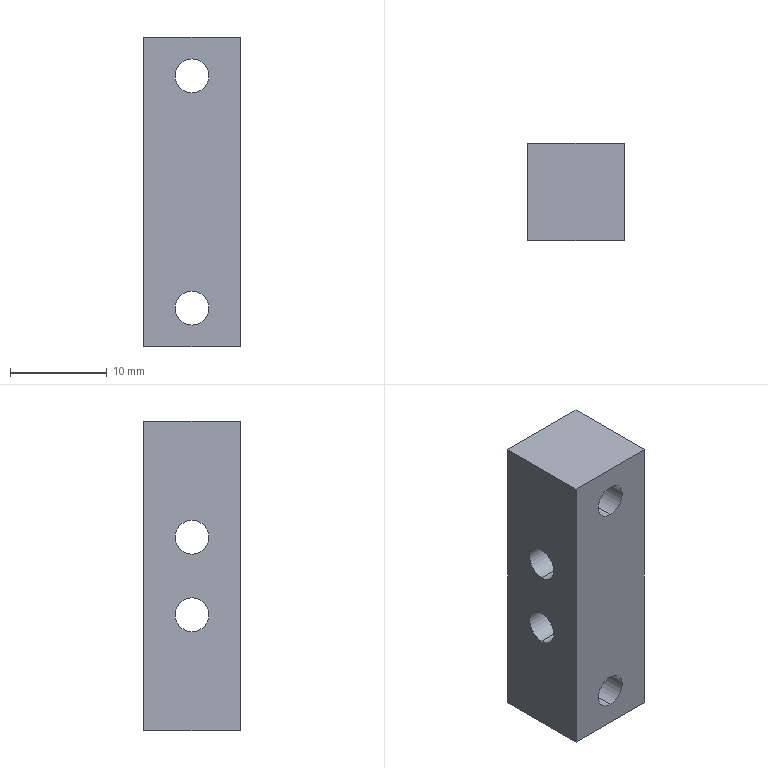Part | SolidWorks | features BaseBody 1 | 1 solid | 14 faces | box 10 x 10 x 32 mm | volume 2815 mm3 | cylinder 8 | plane 6 | commonest cylinder face diameters 3.5 x8
STEP:
#1=CARTESIAN_POINT('',(0.,-5.,-13.75));
#2=VERTEX_POINT('',#1);
#3=CARTESIAN_POINT('',(0.,-5.,-10.25));
#4=VERTEX_POINT('',#3);
#5=CARTESIAN_POINT('',(0.,-5.,-12.));
#6=DIRECTION('',(0.,1.,0.));
#7=DIRECTION('',(0.,0.,1.));
#8=AXIS2_PLACEMENT_3D('',#5,#6,#7);
#9=CIRCLE('',#8,1.75);
#10=EDGE_CURVE('',#2,#4,#9,.T.);
#11=ORIENTED_EDGE('',*,*,#10,.F.);
#12=CARTESIAN_POINT('',(0.,5.,-13.75));
#13=VERTEX_POINT('',#12);
#14=CARTESIAN_POINT('',(0.,-5.,-13.75));
#15=DIRECTION('',(0.,1.,0.));
#16=VECTOR('',#15,1000.);
#17=LINE('',#14,#16);
#18=EDGE_CURVE('',#2,#13,#17,.T.);
#19=ORIENTED_EDGE('',*,*,#18,.T.);
#20=CARTESIAN_POINT('',(0.,5.,-10.25));
#21=VERTEX_POINT('',#20);
#22=CARTESIAN_POINT('',(0.,5.,-12.));
#23=DIRECTION('',(0.,1.,0.));
#24=DIRECTION('',(0.,0.,1.));
#25=AXIS2_PLACEMENT_3D('',#22,#23,#24);
#26=CIRCLE('',#25,1.75);
#27=EDGE_CURVE('',#13,#21,#26,.T.);
#28=ORIENTED_EDGE('',*,*,#27,.T.);
#29=CARTESIAN_POINT('',(0.,-5.,-10.25));
#30=DIRECTION('',(0.,1.,0.));
#31=VECTOR('',#30,1000.);
#32=LINE('',#29,#31);
#33=EDGE_CURVE('',#4,#21,#32,.T.);
#34=ORIENTED_EDGE('',*,*,#33,.F.);
#35=EDGE_LOOP('',(#11,#19,#28,#34));
#36=FACE_OUTER_BOUND('',#35,.T.);
#37=CARTESIAN_POINT('',(0.,-5.,-12.));
#38=DIRECTION('',(0.,1.,0.));
#39=DIRECTION('',(0.,0.,1.));
#40=AXIS2_PLACEMENT_3D('',#37,#38,#39);
#41=CYLINDRICAL_SURFACE('',#40,1.75);
#42=ADVANCED_FACE('',(#36),#41,.F.);
#43=CARTESIAN_POINT('',(0.,-5.,10.25));
#44=VERTEX_POINT('',#43);
#45=CARTESIAN_POINT('',(0.,-5.,13.75));
#46=VERTEX_POINT('',#45);
#47=CARTESIAN_POINT('',(0.,-5.,12.));
#48=DIRECTION('',(0.,1.,0.));
#49=DIRECTION('',(0.,0.,1.));
#50=AXIS2_PLACEMENT_3D('',#47,#48,#49);
#51=CIRCLE('',#50,1.75);
#52=EDGE_CURVE('',#44,#46,#51,.T.);
#53=ORIENTED_EDGE('',*,*,#52,.F.);
#54=CARTESIAN_POINT('',(0.,5.,10.25));
#55=VERTEX_POINT('',#54);
#56=CARTESIAN_POINT('',(0.,-5.,10.25));
#57=DIRECTION('',(0.,1.,0.));
#58=VECTOR('',#57,1000.);
#59=LINE('',#56,#58);
#60=EDGE_CURVE('',#44,#55,#59,.T.);
#61=ORIENTED_EDGE('',*,*,#60,.T.);
#62=CARTESIAN_POINT('',(0.,5.,13.75));
#63=VERTEX_POINT('',#62);
#64=CARTESIAN_POINT('',(0.,5.,12.));
#65=DIRECTION('',(0.,1.,0.));
#66=DIRECTION('',(0.,0.,1.));
#67=AXIS2_PLACEMENT_3D('',#64,#65,#66);
#68=CIRCLE('',#67,1.75);
#69=EDGE_CURVE('',#55,#63,#68,.T.);
#70=ORIENTED_EDGE('',*,*,#69,.T.);
#71=CARTESIAN_POINT('',(0.,-5.,13.75));
#72=DIRECTION('',(0.,1.,0.));
#73=VECTOR('',#72,1000.);
#74=LINE('',#71,#73);
#75=EDGE_CURVE('',#46,#63,#74,.T.);
#76=ORIENTED_EDGE('',*,*,#75,.F.);
#77=EDGE_LOOP('',(#53,#61,#70,#76));
#78=FACE_OUTER_BOUND('',#77,.T.);
#79=CARTESIAN_POINT('',(0.,-5.,12.));
#80=DIRECTION('',(0.,1.,0.));
#81=DIRECTION('',(0.,0.,1.));
#82=AXIS2_PLACEMENT_3D('',#79,#80,#81);
#83=CYLINDRICAL_SURFACE('',#82,1.75);
#84=ADVANCED_FACE('',(#78),#83,.F.);
#85=CARTESIAN_POINT('',(-5.,0.,-2.25));
#86=VERTEX_POINT('',#85);
#87=CARTESIAN_POINT('',(-5.,0.,-5.75));
#88=VERTEX_POINT('',#87);
#89=CARTESIAN_POINT('',(-5.,0.,-4.));
#90=DIRECTION('',(1.,0.,0.));
#91=DIRECTION('',(0.,0.,-1.));
#92=AXIS2_PLACEMENT_3D('',#89,#90,#91);
#93=CIRCLE('',#92,1.75);
#94=EDGE_CURVE('',#86,#88,#93,.T.);
#95=ORIENTED_EDGE('',*,*,#94,.F.);
#96=CARTESIAN_POINT('',(5.,0.,-2.25));
#97=VERTEX_POINT('',#96);
#98=CARTESIAN_POINT('',(-5.,0.,-2.25));
#99=DIRECTION('',(1.,0.,0.));
#100=VECTOR('',#99,1000.);
#101=LINE('',#98,#100);
#102=EDGE_CURVE('',#86,#97,#101,.T.);
#103=ORIENTED_EDGE('',*,*,#102,.T.);
#104=CARTESIAN_POINT('',(5.,0.,-5.75));
#105=VERTEX_POINT('',#104);
#106=CARTESIAN_POINT('',(5.,0.,-4.));
#107=DIRECTION('',(1.,0.,0.));
#108=DIRECTION('',(0.,0.,-1.));
#109=AXIS2_PLACEMENT_3D('',#106,#107,#108);
#110=CIRCLE('',#109,1.75);
#111=EDGE_CURVE('',#97,#105,#110,.T.);
#112=ORIENTED_EDGE('',*,*,#111,.T.);
#113=CARTESIAN_POINT('',(-5.,0.,-5.75));
#114=DIRECTION('',(1.,0.,0.));
#115=VECTOR('',#114,1000.);
#116=LINE('',#113,#115);
#117=EDGE_CURVE('',#88,#105,#116,.T.);
#118=ORIENTED_EDGE('',*,*,#117,.F.);
#119=EDGE_LOOP('',(#95,#103,#112,#118));
#120=FACE_OUTER_BOUND('',#119,.T.);
#121=CARTESIAN_POINT('',(-5.,0.,-4.));
#122=DIRECTION('',(1.,0.,0.));
#123=DIRECTION('',(0.,0.,-1.));
#124=AXIS2_PLACEMENT_3D('',#121,#122,#123);
#125=CYLINDRICAL_SURFACE('',#124,1.75);
#126=ADVANCED_FACE('',(#120),#125,.F.);
#127=CARTESIAN_POINT('',(-5.,0.,5.75));
#128=VERTEX_POINT('',#127);
#129=CARTESIAN_POINT('',(-5.,0.,2.25));
#130=VERTEX_POINT('',#129);
#131=CARTESIAN_POINT('',(-5.,0.,4.));
#132=DIRECTION('',(1.,0.,0.));
#133=DIRECTION('',(0.,0.,-1.));
#134=AXIS2_PLACEMENT_3D('',#131,#132,#133);
#135=CIRCLE('',#134,1.75);
#136=EDGE_CURVE('',#128,#130,#135,.T.);
#137=ORIENTED_EDGE('',*,*,#136,.F.);
#138=CARTESIAN_POINT('',(5.,0.,5.75));
#139=VERTEX_POINT('',#138);
#140=CARTESIAN_POINT('',(-5.,0.,5.75));
#141=DIRECTION('',(1.,0.,0.));
#142=VECTOR('',#141,1000.);
#143=LINE('',#140,#142);
#144=EDGE_CURVE('',#128,#139,#143,.T.);
#145=ORIENTED_EDGE('',*,*,#144,.T.);
#146=CARTESIAN_POINT('',(5.,0.,2.25));
#147=VERTEX_POINT('',#146);
#148=CARTESIAN_POINT('',(5.,0.,4.));
#149=DIRECTION('',(1.,0.,0.));
#150=DIRECTION('',(0.,0.,-1.));
#151=AXIS2_PLACEMENT_3D('',#148,#149,#150);
#152=CIRCLE('',#151,1.75);
#153=EDGE_CURVE('',#139,#147,#152,.T.);
#154=ORIENTED_EDGE('',*,*,#153,.T.);
#155=CARTESIAN_POINT('',(-5.,0.,2.25));
#156=DIRECTION('',(1.,0.,0.));
#157=VECTOR('',#156,1000.);
#158=LINE('',#155,#157);
#159=EDGE_CURVE('',#130,#147,#158,.T.);
#160=ORIENTED_EDGE('',*,*,#159,.F.);
#161=EDGE_LOOP('',(#137,#145,#154,#160));
#162=FACE_OUTER_BOUND('',#161,.T.);
#163=CARTESIAN_POINT('',(-5.,0.,4.));
#164=DIRECTION('',(1.,0.,0.));
#165=DIRECTION('',(0.,0.,-1.));
#166=AXIS2_PLACEMENT_3D('',#163,#164,#165);
#167=CYLINDRICAL_SURFACE('',#166,1.75);
#168=ADVANCED_FACE('',(#162),#167,.F.);
#169=CARTESIAN_POINT('',(5.,5.,16.));
#170=VERTEX_POINT('',#169);
#171=CARTESIAN_POINT('',(-5.,5.,16.));
#172=VERTEX_POINT('',#171);
#173=CARTESIAN_POINT('',(5.,5.,16.));
#174=DIRECTION('',(-1.,0.,0.));
#175=VECTOR('',#174,1000.);
#176=LINE('',#173,#175);
#177=EDGE_CURVE('',#170,#172,#176,.T.);
#178=ORIENTED_EDGE('',*,*,#177,.F.);
#179=CARTESIAN_POINT('',(5.,5.,-16.));
#180=VERTEX_POINT('',#179);
#181=CARTESIAN_POINT('',(5.,5.,16.));
#182=DIRECTION('',(0.,0.,1.));
#183=VECTOR('',#182,1000.);
#184=LINE('',#181,#183);
#185=EDGE_CURVE('',#180,#170,#184,.T.);
#186=ORIENTED_EDGE('',*,*,#185,.F.);
#187=CARTESIAN_POINT('',(-5.,5.,-16.));
#188=VERTEX_POINT('',#187);
#189=CARTESIAN_POINT('',(5.,5.,-16.));
#190=DIRECTION('',(1.,0.,0.));
#191=VECTOR('',#190,1000.);
#192=LINE('',#189,#191);
#193=EDGE_CURVE('',#188,#180,#192,.T.);
#194=ORIENTED_EDGE('',*,*,#193,.F.);
#195=CARTESIAN_POINT('',(-5.,5.,16.));
#196=DIRECTION('',(0.,0.,-1.));
#197=VECTOR('',#196,1000.);
#198=LINE('',#195,#197);
#199=EDGE_CURVE('',#172,#188,#198,.T.);
#200=ORIENTED_EDGE('',*,*,#199,.F.);
#201=EDGE_LOOP('',(#178,#186,#194,#200));
#202=FACE_OUTER_BOUND('',#201,.T.);
#203=CARTESIAN_POINT('',(0.,5.,-12.));
#204=DIRECTION('',(0.,1.,0.));
#205=DIRECTION('',(0.,0.,1.));
#206=AXIS2_PLACEMENT_3D('',#203,#204,#205);
#207=CIRCLE('',#206,1.75);
#208=EDGE_CURVE('',#21,#13,#207,.T.);
#209=ORIENTED_EDGE('',*,*,#208,.F.);
#210=ORIENTED_EDGE('',*,*,#27,.F.);
#211=EDGE_LOOP('',(#209,#210));
#212=FACE_BOUND('',#211,.T.);
#213=CARTESIAN_POINT('',(0.,5.,12.));
#214=DIRECTION('',(0.,1.,0.));
#215=DIRECTION('',(0.,0.,1.));
#216=AXIS2_PLACEMENT_3D('',#213,#214,#215);
#217=CIRCLE('',#216,1.75);
#218=EDGE_CURVE('',#63,#55,#217,.T.);
#219=ORIENTED_EDGE('',*,*,#218,.F.);
#220=ORIENTED_EDGE('',*,*,#69,.F.);
#221=EDGE_LOOP('',(#219,#220));
#222=FACE_BOUND('',#221,.T.);
#223=CARTESIAN_POINT('',(5.,5.,16.));
#224=DIRECTION('',(0.,-1.,0.));
#225=DIRECTION('',(0.,0.,-1.));
#226=AXIS2_PLACEMENT_3D('',#223,#224,#225);
#227=PLANE('',#226);
#228=ADVANCED_FACE('',(#202,#212,#222),#227,.F.);
#229=CARTESIAN_POINT('',(-5.,-5.,16.));
#230=VERTEX_POINT('',#229);
#231=CARTESIAN_POINT('',(-5.,0.,16.));
#232=DIRECTION('',(0.,1.,0.));
#233=VECTOR('',#232,1000.);
#234=LINE('',#231,#233);
#235=EDGE_CURVE('',#230,#172,#234,.T.);
#236=ORIENTED_EDGE('',*,*,#235,.T.);
#237=ORIENTED_EDGE('',*,*,#199,.T.);
#238=CARTESIAN_POINT('',(-5.,-5.,-16.));
#239=VERTEX_POINT('',#238);
#240=CARTESIAN_POINT('',(-5.,0.,-16.));
#241=DIRECTION('',(0.,-1.,0.));
#242=VECTOR('',#241,1000.);
#243=LINE('',#240,#242);
#244=EDGE_CURVE('',#188,#239,#243,.T.);
#245=ORIENTED_EDGE('',*,*,#244,.T.);
#246=CARTESIAN_POINT('',(-5.,-5.,0.));
#247=DIRECTION('',(0.,0.,1.));
#248=VECTOR('',#247,1000.);
#249=LINE('',#246,#248);
#250=EDGE_CURVE('',#239,#230,#249,.T.);
#251=ORIENTED_EDGE('',*,*,#250,.T.);
#252=EDGE_LOOP('',(#236,#237,#245,#251));
#253=FACE_OUTER_BOUND('',#252,.T.);
#254=CARTESIAN_POINT('',(-5.,0.,-4.));
#255=DIRECTION('',(1.,0.,0.));
#256=DIRECTION('',(0.,0.,-1.));
#257=AXIS2_PLACEMENT_3D('',#254,#255,#256);
#258=CIRCLE('',#257,1.75);
#259=EDGE_CURVE('',#88,#86,#258,.T.);
#260=ORIENTED_EDGE('',*,*,#259,.T.);
#261=ORIENTED_EDGE('',*,*,#94,.T.);
#262=EDGE_LOOP('',(#260,#261));
#263=FACE_BOUND('',#262,.T.);
#264=CARTESIAN_POINT('',(-5.,0.,4.));
#265=DIRECTION('',(1.,0.,0.));
#266=DIRECTION('',(0.,0.,-1.));
#267=AXIS2_PLACEMENT_3D('',#264,#265,#266);
#268=CIRCLE('',#267,1.75);
#269=EDGE_CURVE('',#130,#128,#268,.T.);
#270=ORIENTED_EDGE('',*,*,#269,.T.);
#271=ORIENTED_EDGE('',*,*,#136,.T.);
#272=EDGE_LOOP('',(#270,#271));
#273=FACE_BOUND('',#272,.T.);
#274=CARTESIAN_POINT('',(-5.,0.,0.));
#275=DIRECTION('',(-1.,0.,0.));
#276=DIRECTION('',(0.,0.,1.));
#277=AXIS2_PLACEMENT_3D('',#274,#275,#276);
#278=PLANE('',#277);
#279=ADVANCED_FACE('',(#253,#263,#273),#278,.T.);
#280=CARTESIAN_POINT('',(5.,-5.,16.));
#281=VERTEX_POINT('',#280);
#282=CARTESIAN_POINT('',(5.,-5.,16.));
#283=DIRECTION('',(-1.,0.,0.));
#284=VECTOR('',#283,1000.);
#285=LINE('',#282,#284);
#286=EDGE_CURVE('',#281,#230,#285,.T.);
#287=ORIENTED_EDGE('',*,*,#286,.F.);
#288=CARTESIAN_POINT('',(5.,-5.,16.));
#289=DIRECTION('',(0.,-1.,0.));
#290=VECTOR('',#289,1000.);
#291=LINE('',#288,#290);
#292=EDGE_CURVE('',#170,#281,#291,.T.);
#293=ORIENTED_EDGE('',*,*,#292,.F.);
#294=ORIENTED_EDGE('',*,*,#177,.T.);
#295=ORIENTED_EDGE('',*,*,#235,.F.);
#296=EDGE_LOOP('',(#287,#293,#294,#295));
#297=FACE_OUTER_BOUND('',#296,.T.);
#298=CARTESIAN_POINT('',(5.,-5.,16.));
#299=DIRECTION('',(0.,0.,-1.));
#300=DIRECTION('',(-1.,0.,0.));
#301=AXIS2_PLACEMENT_3D('',#298,#299,#300);
#302=PLANE('',#301);
#303=ADVANCED_FACE('',(#297),#302,.F.);
#304=ORIENTED_EDGE('',*,*,#185,.T.);
#305=ORIENTED_EDGE('',*,*,#292,.T.);
#306=CARTESIAN_POINT('',(5.,-5.,-16.));
#307=VERTEX_POINT('',#306);
#308=CARTESIAN_POINT('',(5.,-5.,0.));
#309=DIRECTION('',(0.,0.,1.));
#310=VECTOR('',#309,1000.);
#311=LINE('',#308,#310);
#312=EDGE_CURVE('',#307,#281,#311,.T.);
#313=ORIENTED_EDGE('',*,*,#312,.F.);
#314=CARTESIAN_POINT('',(5.,0.,-16.));
#315=DIRECTION('',(0.,-1.,0.));
#316=VECTOR('',#315,1000.);
#317=LINE('',#314,#316);
#318=EDGE_CURVE('',#180,#307,#317,.T.);
#319=ORIENTED_EDGE('',*,*,#318,.F.);
#320=EDGE_LOOP('',(#304,#305,#313,#319));
#321=FACE_OUTER_BOUND('',#320,.T.);
#322=CARTESIAN_POINT('',(5.,0.,-4.));
#323=DIRECTION('',(1.,0.,0.));
#324=DIRECTION('',(0.,0.,-1.));
#325=AXIS2_PLACEMENT_3D('',#322,#323,#324);
#326=CIRCLE('',#325,1.75);
#327=EDGE_CURVE('',#105,#97,#326,.T.);
#328=ORIENTED_EDGE('',*,*,#327,.F.);
#329=ORIENTED_EDGE('',*,*,#111,.F.);
#330=EDGE_LOOP('',(#328,#329));
#331=FACE_BOUND('',#330,.T.);
#332=CARTESIAN_POINT('',(5.,0.,4.));
#333=DIRECTION('',(1.,0.,0.));
#334=DIRECTION('',(0.,0.,-1.));
#335=AXIS2_PLACEMENT_3D('',#332,#333,#334);
#336=CIRCLE('',#335,1.75);
#337=EDGE_CURVE('',#147,#139,#336,.T.);
#338=ORIENTED_EDGE('',*,*,#337,.F.);
#339=ORIENTED_EDGE('',*,*,#153,.F.);
#340=EDGE_LOOP('',(#338,#339));
#341=FACE_BOUND('',#340,.T.);
#342=CARTESIAN_POINT('',(5.,0.,0.));
#343=DIRECTION('',(-1.,0.,0.));
#344=DIRECTION('',(0.,0.,1.));
#345=AXIS2_PLACEMENT_3D('',#342,#343,#344);
#346=PLANE('',#345);
#347=ADVANCED_FACE('',(#321,#331,#341),#346,.F.);
#348=ORIENTED_EDGE('',*,*,#193,.T.);
#349=ORIENTED_EDGE('',*,*,#318,.T.);
#350=CARTESIAN_POINT('',(5.,-5.,-16.));
#351=DIRECTION('',(1.,0.,0.));
#352=VECTOR('',#351,1000.);
#353=LINE('',#350,#352);
#354=EDGE_CURVE('',#239,#307,#353,.T.);
#355=ORIENTED_EDGE('',*,*,#354,.F.);
#356=ORIENTED_EDGE('',*,*,#244,.F.);
#357=EDGE_LOOP('',(#348,#349,#355,#356));
#358=FACE_OUTER_BOUND('',#357,.T.);
#359=CARTESIAN_POINT('',(5.,-5.,-16.));
#360=DIRECTION('',(0.,0.,1.));
#361=DIRECTION('',(1.,0.,0.));
#362=AXIS2_PLACEMENT_3D('',#359,#360,#361);
#363=PLANE('',#362);
#364=ADVANCED_FACE('',(#358),#363,.F.);
#365=ORIENTED_EDGE('',*,*,#18,.F.);
#366=CARTESIAN_POINT('',(0.,-5.,-12.));
#367=DIRECTION('',(0.,1.,0.));
#368=DIRECTION('',(0.,0.,1.));
#369=AXIS2_PLACEMENT_3D('',#366,#367,#368);
#370=CIRCLE('',#369,1.75);
#371=EDGE_CURVE('',#4,#2,#370,.T.);
#372=ORIENTED_EDGE('',*,*,#371,.F.);
#373=ORIENTED_EDGE('',*,*,#33,.T.);
#374=ORIENTED_EDGE('',*,*,#208,.T.);
#375=EDGE_LOOP('',(#365,#372,#373,#374));
#376=FACE_OUTER_BOUND('',#375,.T.);
#377=CARTESIAN_POINT('',(0.,-5.,-12.));
#378=DIRECTION('',(0.,1.,0.));
#379=DIRECTION('',(0.,0.,1.));
#380=AXIS2_PLACEMENT_3D('',#377,#378,#379);
#381=CYLINDRICAL_SURFACE('',#380,1.75);
#382=ADVANCED_FACE('',(#376),#381,.F.);
#383=ORIENTED_EDGE('',*,*,#60,.F.);
#384=CARTESIAN_POINT('',(0.,-5.,12.));
#385=DIRECTION('',(0.,1.,0.));
#386=DIRECTION('',(0.,0.,1.));
#387=AXIS2_PLACEMENT_3D('',#384,#385,#386);
#388=CIRCLE('',#387,1.75);
#389=EDGE_CURVE('',#46,#44,#388,.T.);
#390=ORIENTED_EDGE('',*,*,#389,.F.);
#391=ORIENTED_EDGE('',*,*,#75,.T.);
#392=ORIENTED_EDGE('',*,*,#218,.T.);
#393=EDGE_LOOP('',(#383,#390,#391,#392));
#394=FACE_OUTER_BOUND('',#393,.T.);
#395=CARTESIAN_POINT('',(0.,-5.,12.));
#396=DIRECTION('',(0.,1.,0.));
#397=DIRECTION('',(0.,0.,1.));
#398=AXIS2_PLACEMENT_3D('',#395,#396,#397);
#399=CYLINDRICAL_SURFACE('',#398,1.75);
#400=ADVANCED_FACE('',(#394),#399,.F.);
#401=ORIENTED_EDGE('',*,*,#354,.T.);
#402=ORIENTED_EDGE('',*,*,#312,.T.);
#403=ORIENTED_EDGE('',*,*,#286,.T.);
#404=ORIENTED_EDGE('',*,*,#250,.F.);
#405=EDGE_LOOP('',(#401,#402,#403,#404));
#406=FACE_OUTER_BOUND('',#405,.T.);
#407=ORIENTED_EDGE('',*,*,#371,.T.);
#408=ORIENTED_EDGE('',*,*,#10,.T.);
#409=EDGE_LOOP('',(#407,#408));
#410=FACE_BOUND('',#409,.T.);
#411=ORIENTED_EDGE('',*,*,#389,.T.);
#412=ORIENTED_EDGE('',*,*,#52,.T.);
#413=EDGE_LOOP('',(#411,#412));
#414=FACE_BOUND('',#413,.T.);
#415=CARTESIAN_POINT('',(5.,-5.,16.));
#416=DIRECTION('',(0.,1.,0.));
#417=DIRECTION('',(0.,0.,1.));
#418=AXIS2_PLACEMENT_3D('',#415,#416,#417);
#419=PLANE('',#418);
#420=ADVANCED_FACE('',(#406,#410,#414),#419,.F.);
#421=ORIENTED_EDGE('',*,*,#102,.F.);
#422=ORIENTED_EDGE('',*,*,#259,.F.);
#423=ORIENTED_EDGE('',*,*,#117,.T.);
#424=ORIENTED_EDGE('',*,*,#327,.T.);
#425=EDGE_LOOP('',(#421,#422,#423,#424));
#426=FACE_OUTER_BOUND('',#425,.T.);
#427=CARTESIAN_POINT('',(-5.,0.,-4.));
#428=DIRECTION('',(1.,0.,0.));
#429=DIRECTION('',(0.,0.,-1.));
#430=AXIS2_PLACEMENT_3D('',#427,#428,#429);
#431=CYLINDRICAL_SURFACE('',#430,1.75);
#432=ADVANCED_FACE('',(#426),#431,.F.);
#433=ORIENTED_EDGE('',*,*,#144,.F.);
#434=ORIENTED_EDGE('',*,*,#269,.F.);
#435=ORIENTED_EDGE('',*,*,#159,.T.);
#436=ORIENTED_EDGE('',*,*,#337,.T.);
#437=EDGE_LOOP('',(#433,#434,#435,#436));
#438=FACE_OUTER_BOUND('',#437,.T.);
#439=CARTESIAN_POINT('',(-5.,0.,4.));
#440=DIRECTION('',(1.,0.,0.));
#441=DIRECTION('',(0.,0.,-1.));
#442=AXIS2_PLACEMENT_3D('',#439,#440,#441);
#443=CYLINDRICAL_SURFACE('',#442,1.75);
#444=ADVANCED_FACE('',(#438),#443,.F.);
#445=CLOSED_SHELL('',(#42,#84,#126,#168,#228,#279,#303,#347,#364,#382,#400,#420,#432,#444));
#446=MANIFOLD_SOLID_BREP('',#445);
#447=CARTESIAN_POINT('',(0.,0.,0.));
#448=DIRECTION('',(0.,0.,1.));
#449=DIRECTION('',(1.,0.,0.));
#450=AXIS2_PLACEMENT_3D('',#447,#448,#449);
#451=(LENGTH_UNIT()NAMED_UNIT(*)SI_UNIT(.MILLI.,.METRE.));
#452=UNCERTAINTY_MEASURE_WITH_UNIT(LENGTH_MEASURE(0.00001),#451,'','');
#453=(NAMED_UNIT(*)PLANE_ANGLE_UNIT()SI_UNIT($,.RADIAN.));
#454=(NAMED_UNIT(*)SI_UNIT($,.STERADIAN.)SOLID_ANGLE_UNIT());
#455=(GEOMETRIC_REPRESENTATION_CONTEXT(3)GLOBAL_UNCERTAINTY_ASSIGNED_CONTEXT((#452))GLOBAL_UNIT_ASSIGNED_CONTEXT((#451,#453,#454))REPRESENTATION_CONTEXT('',''));
#456=ADVANCED_BREP_SHAPE_REPRESENTATION('',(#446,#450),#455);